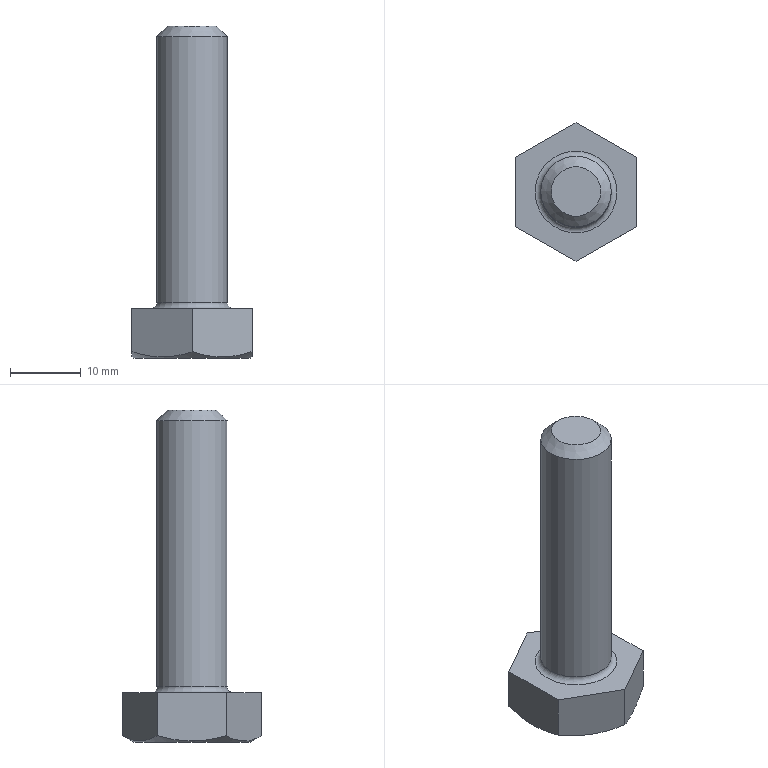Part | STEP file | SI11035_M10 | 1 solid | 13 faces | box 17 x 19.6 x 47 mm | volume 4857 mm3 | plane 9 | cone 2 | cylinder 1 | torus 1 | commonest cylinder face diameters 10 x1
STEP:
#1=CARTESIAN_POINT('',(-5.8,0.,7.));
#2=VERTEX_POINT('',#1);
#3=CARTESIAN_POINT('',(0.,0.,7.));
#4=DIRECTION('',(0.,0.,-1.));
#5=DIRECTION('',(-1.,0.,0.));
#6=AXIS2_PLACEMENT_3D('',#3,#4,#5);
#7=CIRCLE('',#6,5.8);
#8=EDGE_CURVE('',#2,#2,#7,.T.);
#9=ORIENTED_EDGE('',*,*,#8,.T.);
#10=EDGE_LOOP('',(#9));
#11=FACE_BOUND('',#10,.T.);
#12=CARTESIAN_POINT('',(8.5,4.923,7.));
#13=VERTEX_POINT('',#12);
#14=CARTESIAN_POINT('',(0.,9.8,7.));
#15=VERTEX_POINT('',#14);
#16=CARTESIAN_POINT('',(0.,9.8,7.));
#17=DIRECTION('',(-0.8673,0.4977,0.));
#18=VECTOR('',#17,1000.);
#19=LINE('',#16,#18);
#20=EDGE_CURVE('',#13,#15,#19,.T.);
#21=ORIENTED_EDGE('',*,*,#20,.T.);
#22=CARTESIAN_POINT('',(-8.5,4.923,7.));
#23=VERTEX_POINT('',#22);
#24=CARTESIAN_POINT('',(0.,9.8,7.));
#25=DIRECTION('',(-0.8673,-0.4977,0.));
#26=VECTOR('',#25,1000.);
#27=LINE('',#24,#26);
#28=EDGE_CURVE('',#15,#23,#27,.T.);
#29=ORIENTED_EDGE('',*,*,#28,.T.);
#30=CARTESIAN_POINT('',(-8.5,-4.923,7.));
#31=VERTEX_POINT('',#30);
#32=CARTESIAN_POINT('',(-8.5,4.923,7.));
#33=DIRECTION('',(0.,-1.,0.));
#34=VECTOR('',#33,1000.);
#35=LINE('',#32,#34);
#36=EDGE_CURVE('',#23,#31,#35,.T.);
#37=ORIENTED_EDGE('',*,*,#36,.T.);
#38=CARTESIAN_POINT('',(0.,-9.8,7.));
#39=VERTEX_POINT('',#38);
#40=CARTESIAN_POINT('',(0.,-9.8,7.));
#41=DIRECTION('',(0.8673,-0.4977,0.));
#42=VECTOR('',#41,1000.);
#43=LINE('',#40,#42);
#44=EDGE_CURVE('',#31,#39,#43,.T.);
#45=ORIENTED_EDGE('',*,*,#44,.T.);
#46=CARTESIAN_POINT('',(8.5,-4.923,7.));
#47=VERTEX_POINT('',#46);
#48=CARTESIAN_POINT('',(0.,-9.8,7.));
#49=DIRECTION('',(0.8673,0.4977,0.));
#50=VECTOR('',#49,1000.);
#51=LINE('',#48,#50);
#52=EDGE_CURVE('',#39,#47,#51,.T.);
#53=ORIENTED_EDGE('',*,*,#52,.T.);
#54=CARTESIAN_POINT('',(8.5,4.923,7.));
#55=DIRECTION('',(0.,1.,0.));
#56=VECTOR('',#55,1000.);
#57=LINE('',#54,#56);
#58=EDGE_CURVE('',#47,#13,#57,.T.);
#59=ORIENTED_EDGE('',*,*,#58,.T.);
#60=EDGE_LOOP('',(#21,#29,#37,#45,#53,#59));
#61=FACE_OUTER_BOUND('',#60,.T.);
#62=CARTESIAN_POINT('',(8.5,4.923,7.));
#63=DIRECTION('',(0.,0.,-1.));
#64=DIRECTION('',(-1.,0.,0.));
#65=AXIS2_PLACEMENT_3D('',#62,#63,#64);
#66=PLANE('',#65);
#67=ADVANCED_FACE('',(#11,#61),#66,.F.);
#68=CARTESIAN_POINT('',(0.,9.8,0.8949));
#69=VERTEX_POINT('',#68);
#70=CARTESIAN_POINT('',(8.5,4.923,0.9079));
#71=VERTEX_POINT('',#70);
#72=CARTESIAN_POINT('',(0.,9.8,0.8949));
#73=CARTESIAN_POINT('',(0.6942,9.402,0.6649));
#74=CARTESIAN_POINT('',(1.393,9.,0.4757));
#75=CARTESIAN_POINT('',(2.806,8.19,0.2146));
#76=CARTESIAN_POINT('',(3.52,7.78,0.1436));
#77=CARTESIAN_POINT('',(4.604,7.158,0.1447));
#78=CARTESIAN_POINT('',(4.967,6.95,0.1631));
#79=CARTESIAN_POINT('',(5.685,6.538,0.2333));
#80=CARTESIAN_POINT('',(6.041,6.333,0.2852));
#81=CARTESIAN_POINT('',(7.105,5.723,0.4846));
#82=CARTESIAN_POINT('',(7.805,5.321,0.6761));
#83=CARTESIAN_POINT('',(8.5,4.923,0.9079));
#84=B_SPLINE_CURVE_WITH_KNOTS('',3,(#72,#73,#74,#75,#76,#77,#78,#79,#80,#81,#82,#83),.UNSPECIFIED.,.F.,.F.,(4,2,2,2,2,4),(0.000000238,0.002474,0.004949,0.006186,0.007423,0.009897),.UNSPECIFIED.);
#85=EDGE_CURVE('',#69,#71,#84,.T.);
#86=ORIENTED_EDGE('',*,*,#85,.F.);
#87=CARTESIAN_POINT('',(0.,9.8,7.));
#88=DIRECTION('',(0.,0.,-1.));
#89=VECTOR('',#88,1000.);
#90=LINE('',#87,#89);
#91=EDGE_CURVE('',#15,#69,#90,.T.);
#92=ORIENTED_EDGE('',*,*,#91,.F.);
#93=ORIENTED_EDGE('',*,*,#20,.F.);
#94=CARTESIAN_POINT('',(8.5,4.923,7.));
#95=DIRECTION('',(0.,0.,-1.));
#96=VECTOR('',#95,1000.);
#97=LINE('',#94,#96);
#98=EDGE_CURVE('',#13,#71,#97,.T.);
#99=ORIENTED_EDGE('',*,*,#98,.T.);
#100=EDGE_LOOP('',(#86,#92,#93,#99));
#101=FACE_OUTER_BOUND('',#100,.T.);
#102=CARTESIAN_POINT('',(0.,9.8,7.));
#103=DIRECTION('',(-0.4977,-0.8673,0.));
#104=DIRECTION('',(0.8673,-0.4977,0.));
#105=AXIS2_PLACEMENT_3D('',#102,#103,#104);
#106=PLANE('',#105);
#107=ADVANCED_FACE('',(#101),#106,.F.);
#108=CARTESIAN_POINT('',(-8.5,4.923,0.9079));
#109=VERTEX_POINT('',#108);
#110=CARTESIAN_POINT('',(-8.5,4.923,0.9079));
#111=CARTESIAN_POINT('',(-7.806,5.321,0.6764));
#112=CARTESIAN_POINT('',(-7.107,5.722,0.4854));
#113=CARTESIAN_POINT('',(-5.695,6.532,0.2199));
#114=CARTESIAN_POINT('',(-4.982,6.941,0.1462));
#115=CARTESIAN_POINT('',(-3.898,7.563,0.1434));
#116=CARTESIAN_POINT('',(-3.535,7.772,0.1605));
#117=CARTESIAN_POINT('',(-2.816,8.184,0.2282));
#118=CARTESIAN_POINT('',(-2.46,8.389,0.2788));
#119=CARTESIAN_POINT('',(-1.396,8.999,0.475));
#120=CARTESIAN_POINT('',(-0.695,9.401,0.6646));
#121=CARTESIAN_POINT('',(0.,9.8,0.8949));
#122=B_SPLINE_CURVE_WITH_KNOTS('',3,(#110,#111,#112,#113,#114,#115,#116,#117,#118,#119,#120,#121),.UNSPECIFIED.,.F.,.F.,(4,2,2,2,2,4),(0.000000238,0.002474,0.004949,0.006186,0.007423,0.009897),.UNSPECIFIED.);
#123=EDGE_CURVE('',#109,#69,#122,.T.);
#124=ORIENTED_EDGE('',*,*,#123,.F.);
#125=CARTESIAN_POINT('',(-8.5,4.923,7.));
#126=DIRECTION('',(0.,0.,-1.));
#127=VECTOR('',#126,1000.);
#128=LINE('',#125,#127);
#129=EDGE_CURVE('',#23,#109,#128,.T.);
#130=ORIENTED_EDGE('',*,*,#129,.F.);
#131=ORIENTED_EDGE('',*,*,#28,.F.);
#132=ORIENTED_EDGE('',*,*,#91,.T.);
#133=EDGE_LOOP('',(#124,#130,#131,#132));
#134=FACE_OUTER_BOUND('',#133,.T.);
#135=CARTESIAN_POINT('',(0.,9.8,7.));
#136=DIRECTION('',(0.4977,-0.8673,0.));
#137=DIRECTION('',(0.8673,0.4977,0.));
#138=AXIS2_PLACEMENT_3D('',#135,#136,#137);
#139=PLANE('',#138);
#140=ADVANCED_FACE('',(#134),#139,.F.);
#141=CARTESIAN_POINT('',(-8.5,-4.923,0.9079));
#142=VERTEX_POINT('',#141);
#143=CARTESIAN_POINT('',(-8.5,-4.923,0.9079));
#144=CARTESIAN_POINT('',(-8.5,-4.122,0.6762));
#145=CARTESIAN_POINT('',(-8.5,-3.302,0.4818));
#146=CARTESIAN_POINT('',(-8.5,-1.657,0.2159));
#147=CARTESIAN_POINT('',(-8.5,-0.8306,0.1443));
#148=CARTESIAN_POINT('',(-8.5,0.8336,0.1444));
#149=CARTESIAN_POINT('',(-8.5,1.677,0.2182));
#150=CARTESIAN_POINT('',(-8.5,3.321,0.4859));
#151=CARTESIAN_POINT('',(-8.5,4.127,0.6777));
#152=CARTESIAN_POINT('',(-8.5,4.923,0.9079));
#153=B_SPLINE_CURVE_WITH_KNOTS('',3,(#143,#144,#145,#146,#147,#148,#149,#150,#151,#152),.UNSPECIFIED.,.F.,.F.,(4,2,2,2,4),(0.008733,0.01122,0.01372,0.01621,0.0187),.UNSPECIFIED.);
#154=EDGE_CURVE('',#142,#109,#153,.T.);
#155=ORIENTED_EDGE('',*,*,#154,.F.);
#156=CARTESIAN_POINT('',(-8.5,-4.923,7.));
#157=DIRECTION('',(0.,0.,-1.));
#158=VECTOR('',#157,1000.);
#159=LINE('',#156,#158);
#160=EDGE_CURVE('',#31,#142,#159,.T.);
#161=ORIENTED_EDGE('',*,*,#160,.F.);
#162=ORIENTED_EDGE('',*,*,#36,.F.);
#163=ORIENTED_EDGE('',*,*,#129,.T.);
#164=EDGE_LOOP('',(#155,#161,#162,#163));
#165=FACE_OUTER_BOUND('',#164,.T.);
#166=CARTESIAN_POINT('',(-8.5,4.923,7.));
#167=DIRECTION('',(1.,0.,0.));
#168=DIRECTION('',(0.,0.,-1.));
#169=AXIS2_PLACEMENT_3D('',#166,#167,#168);
#170=PLANE('',#169);
#171=ADVANCED_FACE('',(#165),#170,.F.);
#172=CARTESIAN_POINT('',(0.,-9.8,0.8949));
#173=VERTEX_POINT('',#172);
#174=CARTESIAN_POINT('',(0.,-9.8,0.8949));
#175=CARTESIAN_POINT('',(-0.6942,-9.402,0.6649));
#176=CARTESIAN_POINT('',(-1.393,-9.,0.4757));
#177=CARTESIAN_POINT('',(-2.806,-8.19,0.2146));
#178=CARTESIAN_POINT('',(-3.52,-7.78,0.1436));
#179=CARTESIAN_POINT('',(-4.604,-7.158,0.1447));
#180=CARTESIAN_POINT('',(-4.967,-6.95,0.1631));
#181=CARTESIAN_POINT('',(-5.685,-6.538,0.2333));
#182=CARTESIAN_POINT('',(-6.041,-6.333,0.2852));
#183=CARTESIAN_POINT('',(-7.105,-5.723,0.4846));
#184=CARTESIAN_POINT('',(-7.805,-5.321,0.6761));
#185=CARTESIAN_POINT('',(-8.5,-4.923,0.9079));
#186=B_SPLINE_CURVE_WITH_KNOTS('',3,(#174,#175,#176,#177,#178,#179,#180,#181,#182,#183,#184,#185),.UNSPECIFIED.,.F.,.F.,(4,2,2,2,2,4),(0.000000238,0.002474,0.004949,0.006186,0.007423,0.009897),.UNSPECIFIED.);
#187=EDGE_CURVE('',#173,#142,#186,.T.);
#188=ORIENTED_EDGE('',*,*,#187,.F.);
#189=CARTESIAN_POINT('',(0.,-9.8,7.));
#190=DIRECTION('',(0.,0.,-1.));
#191=VECTOR('',#190,1000.);
#192=LINE('',#189,#191);
#193=EDGE_CURVE('',#39,#173,#192,.T.);
#194=ORIENTED_EDGE('',*,*,#193,.F.);
#195=ORIENTED_EDGE('',*,*,#44,.F.);
#196=ORIENTED_EDGE('',*,*,#160,.T.);
#197=EDGE_LOOP('',(#188,#194,#195,#196));
#198=FACE_OUTER_BOUND('',#197,.T.);
#199=CARTESIAN_POINT('',(0.,-9.8,7.));
#200=DIRECTION('',(0.4977,0.8673,0.));
#201=DIRECTION('',(-0.8673,0.4977,0.));
#202=AXIS2_PLACEMENT_3D('',#199,#200,#201);
#203=PLANE('',#202);
#204=ADVANCED_FACE('',(#198),#203,.F.);
#205=CARTESIAN_POINT('',(8.5,-4.923,0.9079));
#206=VERTEX_POINT('',#205);
#207=CARTESIAN_POINT('',(8.5,-4.923,0.9079));
#208=CARTESIAN_POINT('',(7.806,-5.321,0.6764));
#209=CARTESIAN_POINT('',(7.107,-5.722,0.4854));
#210=CARTESIAN_POINT('',(5.695,-6.532,0.2199));
#211=CARTESIAN_POINT('',(4.982,-6.941,0.1462));
#212=CARTESIAN_POINT('',(3.898,-7.563,0.1434));
#213=CARTESIAN_POINT('',(3.535,-7.772,0.1605));
#214=CARTESIAN_POINT('',(2.816,-8.184,0.2282));
#215=CARTESIAN_POINT('',(2.46,-8.389,0.2788));
#216=CARTESIAN_POINT('',(1.396,-8.999,0.475));
#217=CARTESIAN_POINT('',(0.695,-9.401,0.6646));
#218=CARTESIAN_POINT('',(0.,-9.8,0.8949));
#219=B_SPLINE_CURVE_WITH_KNOTS('',3,(#207,#208,#209,#210,#211,#212,#213,#214,#215,#216,#217,#218),.UNSPECIFIED.,.F.,.F.,(4,2,2,2,2,4),(0.000000238,0.002474,0.004949,0.006186,0.007423,0.009897),.UNSPECIFIED.);
#220=EDGE_CURVE('',#206,#173,#219,.T.);
#221=ORIENTED_EDGE('',*,*,#220,.F.);
#222=CARTESIAN_POINT('',(8.5,-4.923,7.));
#223=DIRECTION('',(0.,0.,-1.));
#224=VECTOR('',#223,1000.);
#225=LINE('',#222,#224);
#226=EDGE_CURVE('',#47,#206,#225,.T.);
#227=ORIENTED_EDGE('',*,*,#226,.F.);
#228=ORIENTED_EDGE('',*,*,#52,.F.);
#229=ORIENTED_EDGE('',*,*,#193,.T.);
#230=EDGE_LOOP('',(#221,#227,#228,#229));
#231=FACE_OUTER_BOUND('',#230,.T.);
#232=CARTESIAN_POINT('',(0.,-9.8,7.));
#233=DIRECTION('',(-0.4977,0.8673,0.));
#234=DIRECTION('',(-0.8673,-0.4977,0.));
#235=AXIS2_PLACEMENT_3D('',#232,#233,#234);
#236=PLANE('',#235);
#237=ADVANCED_FACE('',(#231),#236,.F.);
#238=CARTESIAN_POINT('',(8.5,4.923,0.9079));
#239=CARTESIAN_POINT('',(8.5,4.127,0.6777));
#240=CARTESIAN_POINT('',(8.5,3.321,0.4859));
#241=CARTESIAN_POINT('',(8.5,1.677,0.2182));
#242=CARTESIAN_POINT('',(8.5,0.8336,0.1444));
#243=CARTESIAN_POINT('',(8.5,-0.8306,0.1443));
#244=CARTESIAN_POINT('',(8.5,-1.657,0.2159));
#245=CARTESIAN_POINT('',(8.5,-3.302,0.4818));
#246=CARTESIAN_POINT('',(8.5,-4.122,0.6762));
#247=CARTESIAN_POINT('',(8.5,-4.923,0.9079));
#248=B_SPLINE_CURVE_WITH_KNOTS('',3,(#238,#239,#240,#241,#242,#243,#244,#245,#246,#247),.UNSPECIFIED.,.F.,.F.,(4,2,2,2,4),(0.003589,0.006073,0.008558,0.01104,0.01353),.UNSPECIFIED.);
#249=EDGE_CURVE('',#71,#206,#248,.T.);
#250=ORIENTED_EDGE('',*,*,#249,.F.);
#251=ORIENTED_EDGE('',*,*,#98,.F.);
#252=ORIENTED_EDGE('',*,*,#58,.F.);
#253=ORIENTED_EDGE('',*,*,#226,.T.);
#254=EDGE_LOOP('',(#250,#251,#252,#253));
#255=FACE_OUTER_BOUND('',#254,.T.);
#256=CARTESIAN_POINT('',(8.5,4.923,7.));
#257=DIRECTION('',(-1.,0.,0.));
#258=DIRECTION('',(0.,0.,1.));
#259=AXIS2_PLACEMENT_3D('',#256,#257,#258);
#260=PLANE('',#259);
#261=ADVANCED_FACE('',(#255),#260,.F.);
#262=CARTESIAN_POINT('',(8.25,0.,0.));
#263=VERTEX_POINT('',#262);
#264=CARTESIAN_POINT('',(0.,0.,0.));
#265=DIRECTION('',(0.,0.,1.));
#266=DIRECTION('',(1.,0.,0.));
#267=AXIS2_PLACEMENT_3D('',#264,#265,#266);
#268=CIRCLE('',#267,8.25);
#269=EDGE_CURVE('',#263,#263,#268,.T.);
#270=ORIENTED_EDGE('',*,*,#269,.T.);
#271=EDGE_LOOP('',(#270));
#272=FACE_BOUND('',#271,.T.);
#273=ORIENTED_EDGE('',*,*,#85,.T.);
#274=ORIENTED_EDGE('',*,*,#249,.T.);
#275=ORIENTED_EDGE('',*,*,#220,.T.);
#276=ORIENTED_EDGE('',*,*,#187,.T.);
#277=ORIENTED_EDGE('',*,*,#154,.T.);
#278=ORIENTED_EDGE('',*,*,#123,.T.);
#279=EDGE_LOOP('',(#273,#274,#275,#276,#277,#278));
#280=FACE_OUTER_BOUND('',#279,.T.);
#281=CARTESIAN_POINT('',(0.,0.,0.9079));
#282=DIRECTION('',(0.,0.,1.));
#283=DIRECTION('',(1.,0.,0.));
#284=AXIS2_PLACEMENT_3D('',#281,#282,#283);
#285=CONICAL_SURFACE('',#284,9.822,1.047);
#286=ADVANCED_FACE('',(#272,#280),#285,.T.);
#287=ORIENTED_EDGE('',*,*,#269,.F.);
#288=EDGE_LOOP('',(#287));
#289=FACE_OUTER_BOUND('',#288,.T.);
#290=CARTESIAN_POINT('',(8.5,4.923,0.));
#291=DIRECTION('',(0.,0.,-1.));
#292=DIRECTION('',(-1.,0.,0.));
#293=AXIS2_PLACEMENT_3D('',#290,#291,#292);
#294=PLANE('',#293);
#295=ADVANCED_FACE('',(#289),#294,.T.);
#296=CARTESIAN_POINT('',(-5.,0.,7.8));
#297=VERTEX_POINT('',#296);
#298=CARTESIAN_POINT('',(0.,0.,7.8));
#299=DIRECTION('',(0.,0.,1.));
#300=DIRECTION('',(-1.,0.,0.));
#301=AXIS2_PLACEMENT_3D('',#298,#299,#300);
#302=CIRCLE('',#301,5.);
#303=EDGE_CURVE('',#297,#297,#302,.T.);
#304=ORIENTED_EDGE('',*,*,#303,.T.);
#305=EDGE_LOOP('',(#304));
#306=FACE_OUTER_BOUND('',#305,.T.);
#307=CARTESIAN_POINT('',(5.,0.,45.5));
#308=VERTEX_POINT('',#307);
#309=CARTESIAN_POINT('',(0.,0.,45.5));
#310=DIRECTION('',(0.,0.,-1.));
#311=DIRECTION('',(1.,0.,0.));
#312=AXIS2_PLACEMENT_3D('',#309,#310,#311);
#313=CIRCLE('',#312,5.);
#314=EDGE_CURVE('',#308,#308,#313,.T.);
#315=ORIENTED_EDGE('',*,*,#314,.T.);
#316=EDGE_LOOP('',(#315));
#317=FACE_OUTER_BOUND('',#316,.T.);
#318=CARTESIAN_POINT('',(0.,0.,47.));
#319=DIRECTION('',(0.,0.,-1.));
#320=DIRECTION('',(-1.,0.,0.));
#321=AXIS2_PLACEMENT_3D('',#318,#319,#320);
#322=CYLINDRICAL_SURFACE('',#321,5.);
#323=ADVANCED_FACE('',(#306,#317),#322,.T.);
#324=CARTESIAN_POINT('',(3.5,0.,47.));
#325=VERTEX_POINT('',#324);
#326=CARTESIAN_POINT('',(0.,0.,47.));
#327=DIRECTION('',(0.,0.,1.));
#328=DIRECTION('',(1.,0.,0.));
#329=AXIS2_PLACEMENT_3D('',#326,#327,#328);
#330=CIRCLE('',#329,3.5);
#331=EDGE_CURVE('',#325,#325,#330,.T.);
#332=ORIENTED_EDGE('',*,*,#331,.T.);
#333=EDGE_LOOP('',(#332));
#334=FACE_OUTER_BOUND('',#333,.T.);
#335=CARTESIAN_POINT('',(0.,0.,47.));
#336=DIRECTION('',(0.,0.,1.));
#337=DIRECTION('',(1.,0.,0.));
#338=AXIS2_PLACEMENT_3D('',#335,#336,#337);
#339=PLANE('',#338);
#340=ADVANCED_FACE('',(#334),#339,.T.);
#341=ORIENTED_EDGE('',*,*,#314,.F.);
#342=EDGE_LOOP('',(#341));
#343=FACE_OUTER_BOUND('',#342,.T.);
#344=ORIENTED_EDGE('',*,*,#331,.F.);
#345=EDGE_LOOP('',(#344));
#346=FACE_BOUND('',#345,.T.);
#347=CARTESIAN_POINT('',(0.,0.,47.));
#348=DIRECTION('',(0.,0.,-1.));
#349=DIRECTION('',(-1.,0.,0.));
#350=AXIS2_PLACEMENT_3D('',#347,#348,#349);
#351=CONICAL_SURFACE('',#350,3.5,0.7854);
#352=ADVANCED_FACE('',(#343,#346),#351,.T.);
#353=ORIENTED_EDGE('',*,*,#8,.F.);
#354=EDGE_LOOP('',(#353));
#355=FACE_OUTER_BOUND('',#354,.T.);
#356=ORIENTED_EDGE('',*,*,#303,.F.);
#357=EDGE_LOOP('',(#356));
#358=FACE_OUTER_BOUND('',#357,.T.);
#359=CARTESIAN_POINT('',(0.,0.,7.8));
#360=DIRECTION('',(0.,0.,-1.));
#361=DIRECTION('',(-1.,0.,0.));
#362=AXIS2_PLACEMENT_3D('',#359,#360,#361);
#363=TOROIDAL_SURFACE('',#362,5.8,0.8);
#364=ADVANCED_FACE('',(#355,#358),#363,.F.);
#365=CLOSED_SHELL('',(#67,#107,#140,#171,#204,#237,#261,#286,#295,#323,#340,#352,#364));
#366=MANIFOLD_SOLID_BREP('',#365);
#367=CARTESIAN_POINT('',(0.,0.,0.));
#368=DIRECTION('',(0.,0.,1.));
#369=DIRECTION('',(1.,0.,0.));
#370=AXIS2_PLACEMENT_3D('',#367,#368,#369);
#371=(LENGTH_UNIT()NAMED_UNIT(*)SI_UNIT(.MILLI.,.METRE.));
#372=UNCERTAINTY_MEASURE_WITH_UNIT(LENGTH_MEASURE(0.00001),#371,'','');
#373=(NAMED_UNIT(*)PLANE_ANGLE_UNIT()SI_UNIT($,.RADIAN.));
#374=(NAMED_UNIT(*)SI_UNIT($,.STERADIAN.)SOLID_ANGLE_UNIT());
#375=(GEOMETRIC_REPRESENTATION_CONTEXT(3)GLOBAL_UNCERTAINTY_ASSIGNED_CONTEXT((#372))GLOBAL_UNIT_ASSIGNED_CONTEXT((#371,#373,#374))REPRESENTATION_CONTEXT('',''));
#376=ADVANCED_BREP_SHAPE_REPRESENTATION('',(#366,#370),#375);